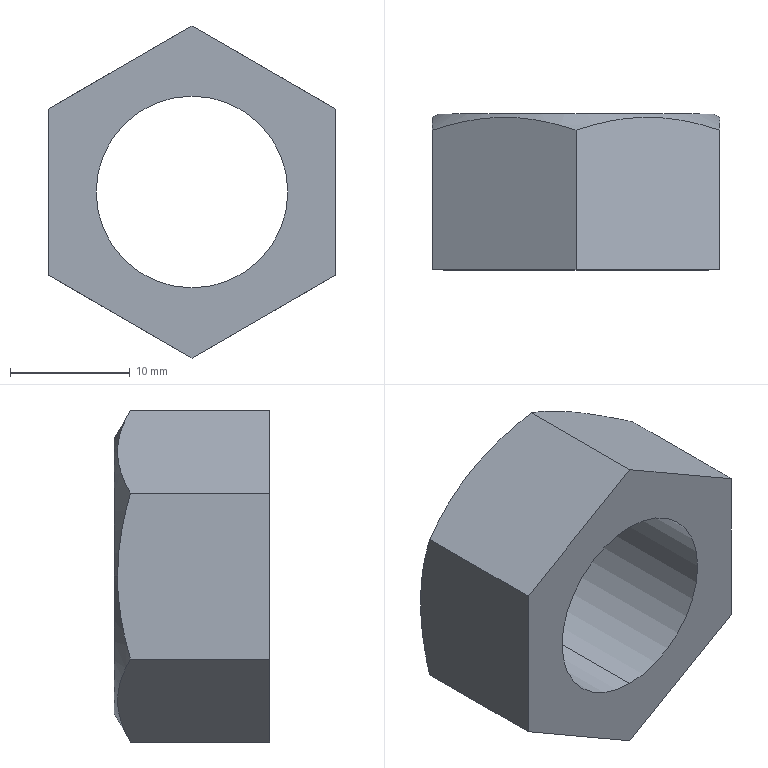Part | STEP file | NN42-M16 | 1 solid | 12 faces | box 24 x 13 x 27.713 mm | volume 3837 mm3 | plane 8 | cylinder 2 | cone 2 | commonest cylinder face diameters 16 x2
STEP:
#1=CARTESIAN_POINT('',(0.,0.,0.));
#2=DIRECTION('',(0.,0.,1.));
#3=DIRECTION('',(1.,0.,0.));
#4=AXIS2_PLACEMENT_3D('',#1,#2,#3);
#5=CARTESIAN_POINT('',(0.,13.,-8.));
#6=VERTEX_POINT('',#5);
#7=CARTESIAN_POINT('',(0.,0.,-8.));
#8=VERTEX_POINT('',#7);
#9=CARTESIAN_POINT('',(0.,13.,-8.));
#10=DIRECTION('',(0.,-1.,0.));
#11=VECTOR('',#10,1.);
#12=LINE('',#9,#11);
#13=CARTESIAN_POINT('',(0.,13.,0.));
#14=DIRECTION('',(0.,-1.,0.));
#15=DIRECTION('',(0.,0.,-1.));
#16=AXIS2_PLACEMENT_3D('',#13,#14,#15);
#17=CYLINDRICAL_SURFACE('',#16,8.);
#18=CARTESIAN_POINT('',(6.283,0.));
#19=DIRECTION('',(0.,1.));
#20=VECTOR('',#19,1.);
#21=LINE('',#18,#20);
#22=(GEOMETRIC_REPRESENTATION_CONTEXT(2)PARAMETRIC_REPRESENTATION_CONTEXT()REPRESENTATION_CONTEXT('',''));
#23=DEFINITIONAL_REPRESENTATION('',(#21),#22);
#24=PCURVE('',#17,#23);
#25=CARTESIAN_POINT('',(0.,13.,0.));
#26=DIRECTION('',(0.,-1.,0.));
#27=DIRECTION('',(0.,0.,-1.));
#28=AXIS2_PLACEMENT_3D('',#25,#26,#27);
#29=CYLINDRICAL_SURFACE('',#28,8.);
#30=CARTESIAN_POINT('',(0.,0.));
#31=DIRECTION('',(0.,1.));
#32=VECTOR('',#31,1.);
#33=LINE('',#30,#32);
#34=(GEOMETRIC_REPRESENTATION_CONTEXT(2)PARAMETRIC_REPRESENTATION_CONTEXT()REPRESENTATION_CONTEXT('',''));
#35=DEFINITIONAL_REPRESENTATION('',(#33),#34);
#36=PCURVE('',#29,#35);
#37=SURFACE_CURVE('',#12,(#24,#36),.PCURVE_S1.);
#38=EDGE_CURVE('',#6,#8,#37,.T.);
#39=ORIENTED_EDGE('',*,*,#38,.T.);
#40=CARTESIAN_POINT('',(0.,0.,8.));
#41=VERTEX_POINT('',#40);
#42=CARTESIAN_POINT('',(0.,0.,0.));
#43=DIRECTION('',(0.,1.,0.));
#44=DIRECTION('',(0.,0.,1.));
#45=AXIS2_PLACEMENT_3D('',#42,#43,#44);
#46=CIRCLE('',#45,8.);
#47=CARTESIAN_POINT('',(9.425,13.));
#48=DIRECTION('',(-1.,0.));
#49=VECTOR('',#48,1.);
#50=LINE('',#47,#49);
#51=(GEOMETRIC_REPRESENTATION_CONTEXT(2)PARAMETRIC_REPRESENTATION_CONTEXT()REPRESENTATION_CONTEXT('',''));
#52=DEFINITIONAL_REPRESENTATION('',(#50),#51);
#53=PCURVE('',#17,#52);
#54=CARTESIAN_POINT('',(0.,0.,0.));
#55=DIRECTION('',(0.,-1.,0.));
#56=DIRECTION('',(0.,0.,1.));
#57=AXIS2_PLACEMENT_3D('',#54,#55,#56);
#58=PLANE('',#57);
#59=CARTESIAN_POINT('',(8.,0.));
#60=CARTESIAN_POINT('',(8.,-13.856));
#61=CARTESIAN_POINT('',(-4.,-6.928));
#62=CARTESIAN_POINT('',(-16.,0.));
#63=CARTESIAN_POINT('',(-4.,6.928));
#64=CARTESIAN_POINT('',(8.,13.856));
#65=CARTESIAN_POINT('',(8.,0.));
#66=(BOUNDED_CURVE()B_SPLINE_CURVE(2,(#59,#60,#61,#62,#63,#64,#65),.UNSPECIFIED.,.T.,.F.)B_SPLINE_CURVE_WITH_KNOTS((1,2,2,2,2,1),(-2.094,0.,2.094,4.189,6.283,8.378),.UNSPECIFIED.)CURVE()GEOMETRIC_REPRESENTATION_ITEM()RATIONAL_B_SPLINE_CURVE((1.,0.5,1.,0.5,1.,0.5,1.))REPRESENTATION_ITEM(''));
#67=(GEOMETRIC_REPRESENTATION_CONTEXT(2)PARAMETRIC_REPRESENTATION_CONTEXT()REPRESENTATION_CONTEXT('',''));
#68=DEFINITIONAL_REPRESENTATION('',(#66),#67);
#69=PCURVE('',#58,#68);
#70=SURFACE_CURVE('',#46,(#53,#69),.PCURVE_S1.);
#71=EDGE_CURVE('',#8,#41,#70,.T.);
#72=ORIENTED_EDGE('',*,*,#71,.T.);
#73=CARTESIAN_POINT('',(0.,13.,8.));
#74=VERTEX_POINT('',#73);
#75=CARTESIAN_POINT('',(0.,13.,8.));
#76=DIRECTION('',(0.,-1.,0.));
#77=VECTOR('',#76,1.);
#78=LINE('',#75,#77);
#79=CARTESIAN_POINT('',(3.142,0.));
#80=DIRECTION('',(0.,1.));
#81=VECTOR('',#80,1.);
#82=LINE('',#79,#81);
#83=(GEOMETRIC_REPRESENTATION_CONTEXT(2)PARAMETRIC_REPRESENTATION_CONTEXT()REPRESENTATION_CONTEXT('',''));
#84=DEFINITIONAL_REPRESENTATION('',(#82),#83);
#85=PCURVE('',#17,#84);
#86=CARTESIAN_POINT('',(3.142,0.));
#87=DIRECTION('',(0.,1.));
#88=VECTOR('',#87,1.);
#89=LINE('',#86,#88);
#90=(GEOMETRIC_REPRESENTATION_CONTEXT(2)PARAMETRIC_REPRESENTATION_CONTEXT()REPRESENTATION_CONTEXT('',''));
#91=DEFINITIONAL_REPRESENTATION('',(#89),#90);
#92=PCURVE('',#29,#91);
#93=SURFACE_CURVE('',#78,(#85,#92),.PCURVE_S1.);
#94=EDGE_CURVE('',#74,#41,#93,.T.);
#95=ORIENTED_EDGE('',*,*,#94,.F.);
#96=CARTESIAN_POINT('',(0.,13.,0.));
#97=DIRECTION('',(0.,-1.,0.));
#98=DIRECTION('',(0.,0.,-1.));
#99=AXIS2_PLACEMENT_3D('',#96,#97,#98);
#100=CIRCLE('',#99,8.);
#101=CARTESIAN_POINT('',(0.,0.));
#102=DIRECTION('',(1.,0.));
#103=VECTOR('',#102,1.);
#104=LINE('',#101,#103);
#105=(GEOMETRIC_REPRESENTATION_CONTEXT(2)PARAMETRIC_REPRESENTATION_CONTEXT()REPRESENTATION_CONTEXT('',''));
#106=DEFINITIONAL_REPRESENTATION('',(#104),#105);
#107=PCURVE('',#17,#106);
#108=CARTESIAN_POINT('',(0.,13.,0.));
#109=DIRECTION('',(0.,1.,0.));
#110=DIRECTION('',(-1.,0.,0.));
#111=AXIS2_PLACEMENT_3D('',#108,#109,#110);
#112=PLANE('',#111);
#113=CARTESIAN_POINT('',(0.,-8.));
#114=CARTESIAN_POINT('',(-13.856,-8.));
#115=CARTESIAN_POINT('',(-6.928,4.));
#116=CARTESIAN_POINT('',(0.,16.));
#117=CARTESIAN_POINT('',(6.928,4.));
#118=CARTESIAN_POINT('',(13.856,-8.));
#119=CARTESIAN_POINT('',(0.,-8.));
#120=(BOUNDED_CURVE()B_SPLINE_CURVE(2,(#113,#114,#115,#116,#117,#118,#119),.UNSPECIFIED.,.T.,.F.)B_SPLINE_CURVE_WITH_KNOTS((1,2,2,2,2,1),(-2.094,0.,2.094,4.189,6.283,8.378),.UNSPECIFIED.)CURVE()GEOMETRIC_REPRESENTATION_ITEM()RATIONAL_B_SPLINE_CURVE((1.,0.5,1.,0.5,1.,0.5,1.))REPRESENTATION_ITEM(''));
#121=(GEOMETRIC_REPRESENTATION_CONTEXT(2)PARAMETRIC_REPRESENTATION_CONTEXT()REPRESENTATION_CONTEXT('',''));
#122=DEFINITIONAL_REPRESENTATION('',(#120),#121);
#123=PCURVE('',#112,#122);
#124=SURFACE_CURVE('',#100,(#107,#123),.PCURVE_S1.);
#125=EDGE_CURVE('',#74,#6,#124,.T.);
#126=ORIENTED_EDGE('',*,*,#125,.T.);
#127=EDGE_LOOP('',(#39,#72,#95,#126));
#128=FACE_BOUND('',#127,.F.);
#129=ADVANCED_FACE('',(#128),#17,.F.);
#130=CARTESIAN_POINT('',(11.5,13.,0.));
#131=VERTEX_POINT('',#130);
#132=CARTESIAN_POINT('',(-11.5,13.,0.));
#133=VERTEX_POINT('',#132);
#134=CARTESIAN_POINT('',(0.,13.,0.));
#135=DIRECTION('',(0.,-1.,0.));
#136=DIRECTION('',(1.,0.,0.));
#137=AXIS2_PLACEMENT_3D('',#134,#135,#136);
#138=CIRCLE('',#137,11.5);
#139=CARTESIAN_POINT('',(0.,13.,0.));
#140=DIRECTION('',(0.,-1.,0.));
#141=DIRECTION('',(1.,0.,0.));
#142=AXIS2_PLACEMENT_3D('',#139,#140,#141);
#143=CONICAL_SURFACE('',#142,11.5,1.047);
#144=CARTESIAN_POINT('',(0.,0.));
#145=DIRECTION('',(1.,0.));
#146=VECTOR('',#145,1.);
#147=LINE('',#144,#146);
#148=(GEOMETRIC_REPRESENTATION_CONTEXT(2)PARAMETRIC_REPRESENTATION_CONTEXT()REPRESENTATION_CONTEXT('',''));
#149=DEFINITIONAL_REPRESENTATION('',(#147),#148);
#150=PCURVE('',#143,#149);
#151=CARTESIAN_POINT('',(-11.5,0.));
#152=CARTESIAN_POINT('',(-11.5,19.919));
#153=CARTESIAN_POINT('',(5.75,9.959));
#154=CARTESIAN_POINT('',(23.,0.));
#155=CARTESIAN_POINT('',(5.75,-9.959));
#156=CARTESIAN_POINT('',(-11.5,-19.919));
#157=CARTESIAN_POINT('',(-11.5,0.));
#158=(BOUNDED_CURVE()B_SPLINE_CURVE(2,(#151,#152,#153,#154,#155,#156,#157),.UNSPECIFIED.,.T.,.F.)B_SPLINE_CURVE_WITH_KNOTS((1,2,2,2,2,1),(-2.094,0.,2.094,4.189,6.283,8.378),.UNSPECIFIED.)CURVE()GEOMETRIC_REPRESENTATION_ITEM()RATIONAL_B_SPLINE_CURVE((1.,0.5,1.,0.5,1.,0.5,1.))REPRESENTATION_ITEM(''));
#159=(GEOMETRIC_REPRESENTATION_CONTEXT(2)PARAMETRIC_REPRESENTATION_CONTEXT()REPRESENTATION_CONTEXT('',''));
#160=DEFINITIONAL_REPRESENTATION('',(#158),#159);
#161=PCURVE('',#112,#160);
#162=SURFACE_CURVE('',#138,(#150,#161),.PCURVE_S1.);
#163=EDGE_CURVE('',#131,#133,#162,.T.);
#164=ORIENTED_EDGE('',*,*,#163,.T.);
#165=CARTESIAN_POINT('',(-12.,12.711,0.));
#166=VERTEX_POINT('',#165);
#167=CARTESIAN_POINT('',(-11.5,13.,0.));
#168=DIRECTION('',(-0.866,-0.5,0.));
#169=VECTOR('',#168,1.);
#170=LINE('',#167,#169);
#171=CARTESIAN_POINT('',(3.142,0.));
#172=DIRECTION('',(0.,1.));
#173=VECTOR('',#172,1.);
#174=LINE('',#171,#173);
#175=(GEOMETRIC_REPRESENTATION_CONTEXT(2)PARAMETRIC_REPRESENTATION_CONTEXT()REPRESENTATION_CONTEXT('',''));
#176=DEFINITIONAL_REPRESENTATION('',(#174),#175);
#177=PCURVE('',#143,#176);
#178=CARTESIAN_POINT('',(0.,13.,0.));
#179=DIRECTION('',(0.,-1.,0.));
#180=DIRECTION('',(1.,0.,0.));
#181=AXIS2_PLACEMENT_3D('',#178,#179,#180);
#182=CONICAL_SURFACE('',#181,11.5,1.047);
#183=CARTESIAN_POINT('',(3.142,0.));
#184=DIRECTION('',(0.,1.));
#185=VECTOR('',#184,1.);
#186=LINE('',#183,#185);
#187=(GEOMETRIC_REPRESENTATION_CONTEXT(2)PARAMETRIC_REPRESENTATION_CONTEXT()REPRESENTATION_CONTEXT('',''));
#188=DEFINITIONAL_REPRESENTATION('',(#186),#187);
#189=PCURVE('',#182,#188);
#190=SURFACE_CURVE('',#170,(#177,#189),.PCURVE_S1.);
#191=EDGE_CURVE('',#133,#166,#190,.T.);
#192=ORIENTED_EDGE('',*,*,#191,.T.);
#193=CARTESIAN_POINT('',(-12.,11.64,6.928));
#194=VERTEX_POINT('',#193);
#195=CARTESIAN_POINT('',(-12.,11.64,6.928));
#196=CARTESIAN_POINT('',(-12.,11.965,5.8));
#197=CARTESIAN_POINT('',(-12.,12.235,4.661));
#198=CARTESIAN_POINT('',(-12.,12.608,2.355));
#199=CARTESIAN_POINT('',(-12.,12.711,1.186));
#200=CARTESIAN_POINT('',(-12.,12.711,0.));
#201=B_SPLINE_CURVE_WITH_KNOTS('',3,(#195,#196,#197,#198,#199,#200),.UNSPECIFIED.,.F.,.F.,(4,2,4),(0.01512,0.01865,0.02217),.UNSPECIFIED.);
#202=CARTESIAN_POINT('',(2.618,1.36));
#203=CARTESIAN_POINT('',(2.624,1.331));
#204=CARTESIAN_POINT('',(2.637,1.273));
#205=CARTESIAN_POINT('',(2.657,1.188));
#206=CARTESIAN_POINT('',(2.678,1.107));
#207=CARTESIAN_POINT('',(2.699,1.028));
#208=CARTESIAN_POINT('',(2.72,0.9532));
#209=CARTESIAN_POINT('',(2.742,0.8815));
#210=CARTESIAN_POINT('',(2.764,0.8133));
#211=CARTESIAN_POINT('',(2.787,0.7487));
#212=CARTESIAN_POINT('',(2.81,0.6879));
#213=CARTESIAN_POINT('',(2.833,0.6309));
#214=CARTESIAN_POINT('',(2.857,0.5779));
#215=CARTESIAN_POINT('',(2.881,0.529));
#216=CARTESIAN_POINT('',(2.906,0.4843));
#217=CARTESIAN_POINT('',(2.931,0.444));
#218=CARTESIAN_POINT('',(2.957,0.408));
#219=CARTESIAN_POINT('',(2.982,0.3766));
#220=CARTESIAN_POINT('',(3.008,0.3498));
#221=CARTESIAN_POINT('',(3.035,0.3277));
#222=CARTESIAN_POINT('',(3.061,0.3104));
#223=CARTESIAN_POINT('',(3.088,0.2979));
#224=CARTESIAN_POINT('',(3.115,0.2904));
#225=CARTESIAN_POINT('',(3.133,0.2887));
#226=CARTESIAN_POINT('',(3.142,0.2887));
#227=B_SPLINE_CURVE_WITH_KNOTS('',3,(#202,#203,#204,#205,#206,#207,#208,#209,#210,#211,#212,#213,#214,#215,#216,#217,#218,#219,#220,#221,#222,#223,#224,#225,#226),.UNSPECIFIED.,.F.,.F.,(4,1,1,1,1,1,1,1,1,1,1,1,1,1,1,1,1,1,1,1,1,1,4),(0.01512,0.01544,0.01576,0.01608,0.0164,0.01672,0.01705,0.01737,0.01769,0.01801,0.01833,0.01865,0.01897,0.01929,0.01961,0.01993,0.02025,0.02057,0.02089,0.02121,0.02153,0.02185,0.02217),.QUASI_UNIFORM_KNOTS.);
#228=(GEOMETRIC_REPRESENTATION_CONTEXT(2)PARAMETRIC_REPRESENTATION_CONTEXT()REPRESENTATION_CONTEXT('',''));
#229=DEFINITIONAL_REPRESENTATION('',(#227),#228);
#230=PCURVE('',#143,#229);
#231=CARTESIAN_POINT('',(-12.,11.64,6.928));
#232=DIRECTION('',(1.,0.,0.));
#233=DIRECTION('',(0.,0.,1.));
#234=AXIS2_PLACEMENT_3D('',#231,#232,#233);
#235=PLANE('',#234);
#236=CARTESIAN_POINT('',(0.,0.));
#237=CARTESIAN_POINT('',(-1.129,-0.3258));
#238=CARTESIAN_POINT('',(-2.267,-0.595));
#239=CARTESIAN_POINT('',(-4.574,-0.9687));
#240=CARTESIAN_POINT('',(-5.742,-1.072));
#241=CARTESIAN_POINT('',(-6.928,-1.072));
#242=B_SPLINE_CURVE_WITH_KNOTS('',3,(#236,#237,#238,#239,#240,#241),.UNSPECIFIED.,.F.,.F.,(4,2,4),(0.01512,0.01865,0.02217),.UNSPECIFIED.);
#243=(GEOMETRIC_REPRESENTATION_CONTEXT(2)PARAMETRIC_REPRESENTATION_CONTEXT()REPRESENTATION_CONTEXT('',''));
#244=DEFINITIONAL_REPRESENTATION('',(#242),#243);
#245=PCURVE('',#235,#244);
#246=SURFACE_CURVE('',#201,(#230,#245),.PCURVE_S1.);
#247=EDGE_CURVE('',#194,#166,#246,.T.);
#248=ORIENTED_EDGE('',*,*,#247,.F.);
#249=CARTESIAN_POINT('',(0.,11.64,13.856));
#250=VERTEX_POINT('',#249);
#251=CARTESIAN_POINT('',(0.,11.64,13.856));
#252=CARTESIAN_POINT('',(-0.9797,11.966,13.291));
#253=CARTESIAN_POINT('',(-1.967,12.235,12.721));
#254=CARTESIAN_POINT('',(-3.961,12.608,11.57));
#255=CARTESIAN_POINT('',(-4.968,12.711,10.988));
#256=CARTESIAN_POINT('',(-6.499,12.712,10.104));
#257=CARTESIAN_POINT('',(-7.011,12.687,9.809));
#258=CARTESIAN_POINT('',(-8.025,12.589,9.223));
#259=CARTESIAN_POINT('',(-8.528,12.516,8.933));
#260=CARTESIAN_POINT('',(-10.03,12.236,8.066));
#261=CARTESIAN_POINT('',(-11.019,11.966,7.495));
#262=CARTESIAN_POINT('',(-12.,11.64,6.928));
#263=B_SPLINE_CURVE_WITH_KNOTS('',3,(#251,#252,#253,#254,#255,#256,#257,#258,#259,#260,#261,#262),.UNSPECIFIED.,.F.,.F.,(4,2,2,2,2,4),(0.000000238,0.003499,0.006997,0.008747,0.0105,0.01399),.UNSPECIFIED.);
#264=CARTESIAN_POINT('',(1.571,1.36));
#265=CARTESIAN_POINT('',(1.584,1.301));
#266=CARTESIAN_POINT('',(1.61,1.186));
#267=CARTESIAN_POINT('',(1.651,1.026));
#268=CARTESIAN_POINT('',(1.694,0.8791));
#269=CARTESIAN_POINT('',(1.739,0.7463));
#270=CARTESIAN_POINT('',(1.786,0.6286));
#271=CARTESIAN_POINT('',(1.834,0.5268));
#272=CARTESIAN_POINT('',(1.884,0.4418));
#273=CARTESIAN_POINT('',(1.935,0.3746));
#274=CARTESIAN_POINT('',(1.987,0.3257));
#275=CARTESIAN_POINT('',(2.04,0.2957));
#276=CARTESIAN_POINT('',(2.093,0.2854));
#277=CARTESIAN_POINT('',(2.147,0.2949));
#278=CARTESIAN_POINT('',(2.2,0.3243));
#279=CARTESIAN_POINT('',(2.253,0.373));
#280=CARTESIAN_POINT('',(2.304,0.4403));
#281=CARTESIAN_POINT('',(2.354,0.5253));
#282=CARTESIAN_POINT('',(2.402,0.6273));
#283=CARTESIAN_POINT('',(2.449,0.7452));
#284=CARTESIAN_POINT('',(2.494,0.8783));
#285=CARTESIAN_POINT('',(2.537,1.026));
#286=CARTESIAN_POINT('',(2.579,1.186));
#287=CARTESIAN_POINT('',(2.605,1.301));
#288=CARTESIAN_POINT('',(2.618,1.36));
#289=B_SPLINE_CURVE_WITH_KNOTS('',3,(#264,#265,#266,#267,#268,#269,#270,#271,#272,#273,#274,#275,#276,#277,#278,#279,#280,#281,#282,#283,#284,#285,#286,#287,#288),.UNSPECIFIED.,.F.,.F.,(4,1,1,1,1,1,1,1,1,1,1,1,1,1,1,1,1,1,1,1,1,1,4),(0.000000238,0.0006363,0.001272,0.001909,0.002545,0.003181,0.003817,0.004453,0.005089,0.005725,0.006361,0.006997,0.007633,0.00827,0.008906,0.009542,0.01018,0.01081,0.01145,0.01209,0.01272,0.01336,0.01399),.QUASI_UNIFORM_KNOTS.);
#290=(GEOMETRIC_REPRESENTATION_CONTEXT(2)PARAMETRIC_REPRESENTATION_CONTEXT()REPRESENTATION_CONTEXT('',''));
#291=DEFINITIONAL_REPRESENTATION('',(#289),#290);
#292=PCURVE('',#143,#291);
#293=CARTESIAN_POINT('',(0.,11.64,13.856));
#294=DIRECTION('',(0.5,0.,-0.866));
#295=DIRECTION('',(0.866,0.,0.5));
#296=AXIS2_PLACEMENT_3D('',#293,#294,#295);
#297=PLANE('',#296);
#298=CARTESIAN_POINT('',(0.,0.));
#299=CARTESIAN_POINT('',(-1.131,-0.3266));
#300=CARTESIAN_POINT('',(-2.271,-0.5957));
#301=CARTESIAN_POINT('',(-4.573,-0.9686));
#302=CARTESIAN_POINT('',(-5.737,-1.071));
#303=CARTESIAN_POINT('',(-7.504,-1.072));
#304=CARTESIAN_POINT('',(-8.096,-1.047));
#305=CARTESIAN_POINT('',(-9.266,-0.9494));
#306=CARTESIAN_POINT('',(-9.848,-0.8769));
#307=CARTESIAN_POINT('',(-11.582,-0.5968));
#308=CARTESIAN_POINT('',(-12.724,-0.327));
#309=CARTESIAN_POINT('',(-13.856,0.));
#310=B_SPLINE_CURVE_WITH_KNOTS('',3,(#298,#299,#300,#301,#302,#303,#304,#305,#306,#307,#308,#309),.UNSPECIFIED.,.F.,.F.,(4,2,2,2,2,4),(0.000000238,0.003499,0.006997,0.008747,0.0105,0.01399),.UNSPECIFIED.);
#311=(GEOMETRIC_REPRESENTATION_CONTEXT(2)PARAMETRIC_REPRESENTATION_CONTEXT()REPRESENTATION_CONTEXT('',''));
#312=DEFINITIONAL_REPRESENTATION('',(#310),#311);
#313=PCURVE('',#297,#312);
#314=SURFACE_CURVE('',#263,(#292,#313),.PCURVE_S1.);
#315=EDGE_CURVE('',#250,#194,#314,.T.);
#316=ORIENTED_EDGE('',*,*,#315,.F.);
#317=CARTESIAN_POINT('',(12.,11.64,6.928));
#318=VERTEX_POINT('',#317);
#319=CARTESIAN_POINT('',(12.,11.64,6.928));
#320=CARTESIAN_POINT('',(11.02,11.966,7.494));
#321=CARTESIAN_POINT('',(10.033,12.235,8.064));
#322=CARTESIAN_POINT('',(8.039,12.608,9.215));
#323=CARTESIAN_POINT('',(7.032,12.711,9.797));
#324=CARTESIAN_POINT('',(5.501,12.712,10.68));
#325=CARTESIAN_POINT('',(4.989,12.687,10.976));
#326=CARTESIAN_POINT('',(3.975,12.589,11.561));
#327=CARTESIAN_POINT('',(3.472,12.516,11.852));
#328=CARTESIAN_POINT('',(1.97,12.236,12.719));
#329=CARTESIAN_POINT('',(0.9809,11.966,13.29));
#330=CARTESIAN_POINT('',(0.,11.64,13.856));
#331=B_SPLINE_CURVE_WITH_KNOTS('',3,(#319,#320,#321,#322,#323,#324,#325,#326,#327,#328,#329,#330),.UNSPECIFIED.,.F.,.F.,(4,2,2,2,2,4),(0.000000238,0.003499,0.006997,0.008747,0.0105,0.01399),.UNSPECIFIED.);
#332=CARTESIAN_POINT('',(0.5236,1.36));
#333=CARTESIAN_POINT('',(0.5365,1.301));
#334=CARTESIAN_POINT('',(0.5628,1.186));
#335=CARTESIAN_POINT('',(0.6041,1.026));
#336=CARTESIAN_POINT('',(0.6472,0.8791));
#337=CARTESIAN_POINT('',(0.6921,0.7463));
#338=CARTESIAN_POINT('',(0.7388,0.6286));
#339=CARTESIAN_POINT('',(0.787,0.5268));
#340=CARTESIAN_POINT('',(0.8367,0.4418));
#341=CARTESIAN_POINT('',(0.8877,0.3746));
#342=CARTESIAN_POINT('',(0.9397,0.3257));
#343=CARTESIAN_POINT('',(0.9926,0.2957));
#344=CARTESIAN_POINT('',(1.046,0.2854));
#345=CARTESIAN_POINT('',(1.1,0.2949));
#346=CARTESIAN_POINT('',(1.153,0.3243));
#347=CARTESIAN_POINT('',(1.205,0.373));
#348=CARTESIAN_POINT('',(1.257,0.4403));
#349=CARTESIAN_POINT('',(1.307,0.5253));
#350=CARTESIAN_POINT('',(1.355,0.6273));
#351=CARTESIAN_POINT('',(1.402,0.7452));
#352=CARTESIAN_POINT('',(1.447,0.8783));
#353=CARTESIAN_POINT('',(1.49,1.026));
#354=CARTESIAN_POINT('',(1.532,1.186));
#355=CARTESIAN_POINT('',(1.558,1.301));
#356=CARTESIAN_POINT('',(1.571,1.36));
#357=B_SPLINE_CURVE_WITH_KNOTS('',3,(#332,#333,#334,#335,#336,#337,#338,#339,#340,#341,#342,#343,#344,#345,#346,#347,#348,#349,#350,#351,#352,#353,#354,#355,#356),.UNSPECIFIED.,.F.,.F.,(4,1,1,1,1,1,1,1,1,1,1,1,1,1,1,1,1,1,1,1,1,1,4),(0.000000238,0.0006363,0.001272,0.001909,0.002545,0.003181,0.003817,0.004453,0.005089,0.005725,0.006361,0.006997,0.007633,0.00827,0.008906,0.009542,0.01018,0.01081,0.01145,0.01209,0.01272,0.01336,0.01399),.QUASI_UNIFORM_KNOTS.);
#358=(GEOMETRIC_REPRESENTATION_CONTEXT(2)PARAMETRIC_REPRESENTATION_CONTEXT()REPRESENTATION_CONTEXT('',''));
#359=DEFINITIONAL_REPRESENTATION('',(#357),#358);
#360=PCURVE('',#143,#359);
#361=CARTESIAN_POINT('',(12.,11.64,6.928));
#362=DIRECTION('',(-0.5,0.,-0.866));
#363=DIRECTION('',(0.866,0.,-0.5));
#364=AXIS2_PLACEMENT_3D('',#361,#362,#363);
#365=PLANE('',#364);
#366=CARTESIAN_POINT('',(0.,0.));
#367=CARTESIAN_POINT('',(-1.131,-0.3266));
#368=CARTESIAN_POINT('',(-2.271,-0.5957));
#369=CARTESIAN_POINT('',(-4.573,-0.9686));
#370=CARTESIAN_POINT('',(-5.737,-1.071));
#371=CARTESIAN_POINT('',(-7.504,-1.072));
#372=CARTESIAN_POINT('',(-8.096,-1.047));
#373=CARTESIAN_POINT('',(-9.266,-0.9494));
#374=CARTESIAN_POINT('',(-9.848,-0.8769));
#375=CARTESIAN_POINT('',(-11.582,-0.5968));
#376=CARTESIAN_POINT('',(-12.724,-0.327));
#377=CARTESIAN_POINT('',(-13.856,0.));
#378=B_SPLINE_CURVE_WITH_KNOTS('',3,(#366,#367,#368,#369,#370,#371,#372,#373,#374,#375,#376,#377),.UNSPECIFIED.,.F.,.F.,(4,2,2,2,2,4),(0.000000238,0.003499,0.006997,0.008747,0.0105,0.01399),.UNSPECIFIED.);
#379=(GEOMETRIC_REPRESENTATION_CONTEXT(2)PARAMETRIC_REPRESENTATION_CONTEXT()REPRESENTATION_CONTEXT('',''));
#380=DEFINITIONAL_REPRESENTATION('',(#378),#379);
#381=PCURVE('',#365,#380);
#382=SURFACE_CURVE('',#331,(#360,#381),.PCURVE_S1.);
#383=EDGE_CURVE('',#318,#250,#382,.T.);
#384=ORIENTED_EDGE('',*,*,#383,.F.);
#385=CARTESIAN_POINT('',(12.,12.711,0.));
#386=VERTEX_POINT('',#385);
#387=CARTESIAN_POINT('',(12.,12.711,0.));
#388=CARTESIAN_POINT('',(12.,12.711,1.186));
#389=CARTESIAN_POINT('',(12.,12.608,2.357));
#390=CARTESIAN_POINT('',(12.,12.234,4.663));
#391=CARTESIAN_POINT('',(12.,11.965,5.801));
#392=CARTESIAN_POINT('',(12.,11.64,6.928));
#393=B_SPLINE_CURVE_WITH_KNOTS('',3,(#387,#388,#389,#390,#391,#392),.UNSPECIFIED.,.F.,.F.,(4,2,4),(0.02217,0.02569,0.02922),.UNSPECIFIED.);
#394=CARTESIAN_POINT('',(0.,0.2887));
#395=CARTESIAN_POINT('',(0.008984,0.2887));
#396=CARTESIAN_POINT('',(0.02693,0.2904));
#397=CARTESIAN_POINT('',(0.05375,0.2979));
#398=CARTESIAN_POINT('',(0.08043,0.3104));
#399=CARTESIAN_POINT('',(0.1069,0.3277));
#400=CARTESIAN_POINT('',(0.1332,0.3499));
#401=CARTESIAN_POINT('',(0.1592,0.3767));
#402=CARTESIAN_POINT('',(0.185,0.4082));
#403=CARTESIAN_POINT('',(0.2104,0.4442));
#404=CARTESIAN_POINT('',(0.2355,0.4846));
#405=CARTESIAN_POINT('',(0.2603,0.5294));
#406=CARTESIAN_POINT('',(0.2846,0.5783));
#407=CARTESIAN_POINT('',(0.3086,0.6313));
#408=CARTESIAN_POINT('',(0.3321,0.6883));
#409=CARTESIAN_POINT('',(0.3552,0.7491));
#410=CARTESIAN_POINT('',(0.3779,0.8137));
#411=CARTESIAN_POINT('',(0.4001,0.8818));
#412=CARTESIAN_POINT('',(0.4218,0.9535));
#413=CARTESIAN_POINT('',(0.4431,1.029));
#414=CARTESIAN_POINT('',(0.464,1.107));
#415=CARTESIAN_POINT('',(0.4843,1.188));
#416=CARTESIAN_POINT('',(0.5042,1.273));
#417=CARTESIAN_POINT('',(0.5172,1.331));
#418=CARTESIAN_POINT('',(0.5236,1.36));
#419=B_SPLINE_CURVE_WITH_KNOTS('',3,(#394,#395,#396,#397,#398,#399,#400,#401,#402,#403,#404,#405,#406,#407,#408,#409,#410,#411,#412,#413,#414,#415,#416,#417,#418),.UNSPECIFIED.,.F.,.F.,(4,1,1,1,1,1,1,1,1,1,1,1,1,1,1,1,1,1,1,1,1,1,4),(0.02217,0.02249,0.02281,0.02313,0.02345,0.02377,0.02409,0.02441,0.02473,0.02505,0.02537,0.02569,0.02601,0.02633,0.02665,0.02697,0.02729,0.02762,0.02794,0.02826,0.02858,0.0289,0.02922),.QUASI_UNIFORM_KNOTS.);
#420=(GEOMETRIC_REPRESENTATION_CONTEXT(2)PARAMETRIC_REPRESENTATION_CONTEXT()REPRESENTATION_CONTEXT('',''));
#421=DEFINITIONAL_REPRESENTATION('',(#419),#420);
#422=PCURVE('',#143,#421);
#423=CARTESIAN_POINT('',(12.,11.64,-6.928));
#424=DIRECTION('',(-1.,0.,0.));
#425=DIRECTION('',(0.,0.,-1.));
#426=AXIS2_PLACEMENT_3D('',#423,#424,#425);
#427=PLANE('',#426);
#428=CARTESIAN_POINT('',(-6.928,-1.072));
#429=CARTESIAN_POINT('',(-8.114,-1.072));
#430=CARTESIAN_POINT('',(-9.285,-0.9684));
#431=CARTESIAN_POINT('',(-11.591,-0.5946));
#432=CARTESIAN_POINT('',(-12.729,-0.3254));
#433=CARTESIAN_POINT('',(-13.856,0.));
#434=B_SPLINE_CURVE_WITH_KNOTS('',3,(#428,#429,#430,#431,#432,#433),.UNSPECIFIED.,.F.,.F.,(4,2,4),(0.02217,0.02569,0.02922),.UNSPECIFIED.);
#435=(GEOMETRIC_REPRESENTATION_CONTEXT(2)PARAMETRIC_REPRESENTATION_CONTEXT()REPRESENTATION_CONTEXT('',''));
#436=DEFINITIONAL_REPRESENTATION('',(#434),#435);
#437=PCURVE('',#427,#436);
#438=SURFACE_CURVE('',#393,(#422,#437),.PCURVE_S1.);
#439=EDGE_CURVE('',#386,#318,#438,.T.);
#440=ORIENTED_EDGE('',*,*,#439,.F.);
#441=CARTESIAN_POINT('',(11.5,13.,0.));
#442=DIRECTION('',(0.866,-0.5,0.));
#443=VECTOR('',#442,1.);
#444=LINE('',#441,#443);
#445=CARTESIAN_POINT('',(0.,0.));
#446=DIRECTION('',(0.,1.));
#447=VECTOR('',#446,1.);
#448=LINE('',#445,#447);
#449=(GEOMETRIC_REPRESENTATION_CONTEXT(2)PARAMETRIC_REPRESENTATION_CONTEXT()REPRESENTATION_CONTEXT('',''));
#450=DEFINITIONAL_REPRESENTATION('',(#448),#449);
#451=PCURVE('',#143,#450);
#452=CARTESIAN_POINT('',(6.283,0.));
#453=DIRECTION('',(0.,1.));
#454=VECTOR('',#453,1.);
#455=LINE('',#452,#454);
#456=(GEOMETRIC_REPRESENTATION_CONTEXT(2)PARAMETRIC_REPRESENTATION_CONTEXT()REPRESENTATION_CONTEXT('',''));
#457=DEFINITIONAL_REPRESENTATION('',(#455),#456);
#458=PCURVE('',#182,#457);
#459=SURFACE_CURVE('',#444,(#451,#458),.PCURVE_S1.);
#460=EDGE_CURVE('',#131,#386,#459,.T.);
#461=ORIENTED_EDGE('',*,*,#460,.F.);
#462=EDGE_LOOP('',(#164,#192,#248,#316,#384,#440,#461));
#463=FACE_BOUND('',#462,.T.);
#464=ADVANCED_FACE('',(#463),#143,.T.);
#465=ORIENTED_EDGE('',*,*,#191,.F.);
#466=CARTESIAN_POINT('',(0.,13.,0.));
#467=DIRECTION('',(0.,-1.,0.));
#468=DIRECTION('',(1.,0.,0.));
#469=AXIS2_PLACEMENT_3D('',#466,#467,#468);
#470=CIRCLE('',#469,11.5);
#471=CARTESIAN_POINT('',(0.,0.));
#472=DIRECTION('',(1.,0.));
#473=VECTOR('',#472,1.);
#474=LINE('',#471,#473);
#475=(GEOMETRIC_REPRESENTATION_CONTEXT(2)PARAMETRIC_REPRESENTATION_CONTEXT()REPRESENTATION_CONTEXT('',''));
#476=DEFINITIONAL_REPRESENTATION('',(#474),#475);
#477=PCURVE('',#182,#476);
#478=CARTESIAN_POINT('',(-11.5,0.));
#479=CARTESIAN_POINT('',(-11.5,19.919));
#480=CARTESIAN_POINT('',(5.75,9.959));
#481=CARTESIAN_POINT('',(23.,0.));
#482=CARTESIAN_POINT('',(5.75,-9.959));
#483=CARTESIAN_POINT('',(-11.5,-19.919));
#484=CARTESIAN_POINT('',(-11.5,0.));
#485=(BOUNDED_CURVE()B_SPLINE_CURVE(2,(#478,#479,#480,#481,#482,#483,#484),.UNSPECIFIED.,.T.,.F.)B_SPLINE_CURVE_WITH_KNOTS((1,2,2,2,2,1),(-2.094,0.,2.094,4.189,6.283,8.378),.UNSPECIFIED.)CURVE()GEOMETRIC_REPRESENTATION_ITEM()RATIONAL_B_SPLINE_CURVE((1.,0.5,1.,0.5,1.,0.5,1.))REPRESENTATION_ITEM(''));
#486=(GEOMETRIC_REPRESENTATION_CONTEXT(2)PARAMETRIC_REPRESENTATION_CONTEXT()REPRESENTATION_CONTEXT('',''));
#487=DEFINITIONAL_REPRESENTATION('',(#485),#486);
#488=PCURVE('',#112,#487);
#489=SURFACE_CURVE('',#470,(#477,#488),.PCURVE_S1.);
#490=EDGE_CURVE('',#133,#131,#489,.T.);
#491=ORIENTED_EDGE('',*,*,#490,.T.);
#492=ORIENTED_EDGE('',*,*,#460,.T.);
#493=CARTESIAN_POINT('',(12.,11.64,-6.928));
#494=VERTEX_POINT('',#493);
#495=CARTESIAN_POINT('',(12.,11.64,-6.928));
#496=CARTESIAN_POINT('',(12.,11.965,-5.8));
#497=CARTESIAN_POINT('',(12.,12.235,-4.661));
#498=CARTESIAN_POINT('',(12.,12.608,-2.355));
#499=CARTESIAN_POINT('',(12.,12.711,-1.186));
#500=CARTESIAN_POINT('',(12.,12.711,0.));
#501=B_SPLINE_CURVE_WITH_KNOTS('',3,(#495,#496,#497,#498,#499,#500),.UNSPECIFIED.,.F.,.F.,(4,2,4),(0.01512,0.01865,0.02217),.UNSPECIFIED.);
#502=CARTESIAN_POINT('',(5.76,1.36));
#503=CARTESIAN_POINT('',(5.766,1.331));
#504=CARTESIAN_POINT('',(5.779,1.273));
#505=CARTESIAN_POINT('',(5.799,1.188));
#506=CARTESIAN_POINT('',(5.819,1.107));
#507=CARTESIAN_POINT('',(5.84,1.028));
#508=CARTESIAN_POINT('',(5.861,0.9532));
#509=CARTESIAN_POINT('',(5.883,0.8815));
#510=CARTESIAN_POINT('',(5.905,0.8133));
#511=CARTESIAN_POINT('',(5.928,0.7487));
#512=CARTESIAN_POINT('',(5.951,0.6879));
#513=CARTESIAN_POINT('',(5.975,0.6309));
#514=CARTESIAN_POINT('',(5.999,0.5779));
#515=CARTESIAN_POINT('',(6.023,0.529));
#516=CARTESIAN_POINT('',(6.048,0.4843));
#517=CARTESIAN_POINT('',(6.073,0.444));
#518=CARTESIAN_POINT('',(6.098,0.408));
#519=CARTESIAN_POINT('',(6.124,0.3766));
#520=CARTESIAN_POINT('',(6.15,0.3498));
#521=CARTESIAN_POINT('',(6.176,0.3277));
#522=CARTESIAN_POINT('',(6.203,0.3104));
#523=CARTESIAN_POINT('',(6.229,0.2979));
#524=CARTESIAN_POINT('',(6.256,0.2904));
#525=CARTESIAN_POINT('',(6.274,0.2887));
#526=CARTESIAN_POINT('',(6.283,0.2887));
#527=B_SPLINE_CURVE_WITH_KNOTS('',3,(#502,#503,#504,#505,#506,#507,#508,#509,#510,#511,#512,#513,#514,#515,#516,#517,#518,#519,#520,#521,#522,#523,#524,#525,#526),.UNSPECIFIED.,.F.,.F.,(4,1,1,1,1,1,1,1,1,1,1,1,1,1,1,1,1,1,1,1,1,1,4),(0.01512,0.01544,0.01576,0.01608,0.0164,0.01672,0.01705,0.01737,0.01769,0.01801,0.01833,0.01865,0.01897,0.01929,0.01961,0.01993,0.02025,0.02057,0.02089,0.02121,0.02153,0.02185,0.02217),.QUASI_UNIFORM_KNOTS.);
#528=(GEOMETRIC_REPRESENTATION_CONTEXT(2)PARAMETRIC_REPRESENTATION_CONTEXT()REPRESENTATION_CONTEXT('',''));
#529=DEFINITIONAL_REPRESENTATION('',(#527),#528);
#530=PCURVE('',#182,#529);
#531=CARTESIAN_POINT('',(0.,0.));
#532=CARTESIAN_POINT('',(-1.129,-0.3258));
#533=CARTESIAN_POINT('',(-2.267,-0.595));
#534=CARTESIAN_POINT('',(-4.574,-0.9687));
#535=CARTESIAN_POINT('',(-5.742,-1.072));
#536=CARTESIAN_POINT('',(-6.928,-1.072));
#537=B_SPLINE_CURVE_WITH_KNOTS('',3,(#531,#532,#533,#534,#535,#536),.UNSPECIFIED.,.F.,.F.,(4,2,4),(0.01512,0.01865,0.02217),.UNSPECIFIED.);
#538=(GEOMETRIC_REPRESENTATION_CONTEXT(2)PARAMETRIC_REPRESENTATION_CONTEXT()REPRESENTATION_CONTEXT('',''));
#539=DEFINITIONAL_REPRESENTATION('',(#537),#538);
#540=PCURVE('',#427,#539);
#541=SURFACE_CURVE('',#501,(#530,#540),.PCURVE_S1.);
#542=EDGE_CURVE('',#494,#386,#541,.T.);
#543=ORIENTED_EDGE('',*,*,#542,.F.);
#544=CARTESIAN_POINT('',(0.,11.64,-13.856));
#545=VERTEX_POINT('',#544);
#546=CARTESIAN_POINT('',(0.,11.64,-13.856));
#547=CARTESIAN_POINT('',(0.9797,11.966,-13.291));
#548=CARTESIAN_POINT('',(1.967,12.235,-12.721));
#549=CARTESIAN_POINT('',(3.961,12.608,-11.57));
#550=CARTESIAN_POINT('',(4.968,12.711,-10.988));
#551=CARTESIAN_POINT('',(6.499,12.712,-10.104));
#552=CARTESIAN_POINT('',(7.011,12.687,-9.809));
#553=CARTESIAN_POINT('',(8.025,12.589,-9.223));
#554=CARTESIAN_POINT('',(8.528,12.516,-8.933));
#555=CARTESIAN_POINT('',(10.03,12.236,-8.066));
#556=CARTESIAN_POINT('',(11.019,11.966,-7.495));
#557=CARTESIAN_POINT('',(12.,11.64,-6.928));
#558=B_SPLINE_CURVE_WITH_KNOTS('',3,(#546,#547,#548,#549,#550,#551,#552,#553,#554,#555,#556,#557),.UNSPECIFIED.,.F.,.F.,(4,2,2,2,2,4),(0.000000238,0.003499,0.006997,0.008747,0.0105,0.01399),.UNSPECIFIED.);
#559=CARTESIAN_POINT('',(4.712,1.36));
#560=CARTESIAN_POINT('',(4.725,1.301));
#561=CARTESIAN_POINT('',(4.752,1.186));
#562=CARTESIAN_POINT('',(4.793,1.026));
#563=CARTESIAN_POINT('',(4.836,0.8791));
#564=CARTESIAN_POINT('',(4.881,0.7463));
#565=CARTESIAN_POINT('',(4.928,0.6286));
#566=CARTESIAN_POINT('',(4.976,0.5268));
#567=CARTESIAN_POINT('',(5.025,0.4418));
#568=CARTESIAN_POINT('',(5.076,0.3746));
#569=CARTESIAN_POINT('',(5.129,0.3257));
#570=CARTESIAN_POINT('',(5.181,0.2957));
#571=CARTESIAN_POINT('',(5.235,0.2854));
#572=CARTESIAN_POINT('',(5.288,0.2949));
#573=CARTESIAN_POINT('',(5.342,0.3243));
#574=CARTESIAN_POINT('',(5.394,0.373));
#575=CARTESIAN_POINT('',(5.445,0.4403));
#576=CARTESIAN_POINT('',(5.495,0.5253));
#577=CARTESIAN_POINT('',(5.544,0.6273));
#578=CARTESIAN_POINT('',(5.591,0.7452));
#579=CARTESIAN_POINT('',(5.636,0.8783));
#580=CARTESIAN_POINT('',(5.679,1.026));
#581=CARTESIAN_POINT('',(5.72,1.186));
#582=CARTESIAN_POINT('',(5.747,1.301));
#583=CARTESIAN_POINT('',(5.76,1.36));
#584=B_SPLINE_CURVE_WITH_KNOTS('',3,(#559,#560,#561,#562,#563,#564,#565,#566,#567,#568,#569,#570,#571,#572,#573,#574,#575,#576,#577,#578,#579,#580,#581,#582,#583),.UNSPECIFIED.,.F.,.F.,(4,1,1,1,1,1,1,1,1,1,1,1,1,1,1,1,1,1,1,1,1,1,4),(0.000000238,0.0006363,0.001272,0.001909,0.002545,0.003181,0.003817,0.004453,0.005089,0.005725,0.006361,0.006997,0.007633,0.00827,0.008906,0.009542,0.01018,0.01081,0.01145,0.01209,0.01272,0.01336,0.01399),.QUASI_UNIFORM_KNOTS.);
#585=(GEOMETRIC_REPRESENTATION_CONTEXT(2)PARAMETRIC_REPRESENTATION_CONTEXT()REPRESENTATION_CONTEXT('',''));
#586=DEFINITIONAL_REPRESENTATION('',(#584),#585);
#587=PCURVE('',#182,#586);
#588=CARTESIAN_POINT('',(0.,11.64,-13.856));
#589=DIRECTION('',(-0.5,0.,0.866));
#590=DIRECTION('',(-0.866,0.,-0.5));
#591=AXIS2_PLACEMENT_3D('',#588,#589,#590);
#592=PLANE('',#591);
#593=CARTESIAN_POINT('',(0.,0.));
#594=CARTESIAN_POINT('',(-1.131,-0.3266));
#595=CARTESIAN_POINT('',(-2.271,-0.5957));
#596=CARTESIAN_POINT('',(-4.573,-0.9686));
#597=CARTESIAN_POINT('',(-5.737,-1.071));
#598=CARTESIAN_POINT('',(-7.504,-1.072));
#599=CARTESIAN_POINT('',(-8.096,-1.047));
#600=CARTESIAN_POINT('',(-9.266,-0.9494));
#601=CARTESIAN_POINT('',(-9.848,-0.8769));
#602=CARTESIAN_POINT('',(-11.582,-0.5968));
#603=CARTESIAN_POINT('',(-12.724,-0.327));
#604=CARTESIAN_POINT('',(-13.856,0.));
#605=B_SPLINE_CURVE_WITH_KNOTS('',3,(#593,#594,#595,#596,#597,#598,#599,#600,#601,#602,#603,#604),.UNSPECIFIED.,.F.,.F.,(4,2,2,2,2,4),(0.000000238,0.003499,0.006997,0.008747,0.0105,0.01399),.UNSPECIFIED.);
#606=(GEOMETRIC_REPRESENTATION_CONTEXT(2)PARAMETRIC_REPRESENTATION_CONTEXT()REPRESENTATION_CONTEXT('',''));
#607=DEFINITIONAL_REPRESENTATION('',(#605),#606);
#608=PCURVE('',#592,#607);
#609=SURFACE_CURVE('',#558,(#587,#608),.PCURVE_S1.);
#610=EDGE_CURVE('',#545,#494,#609,.T.);
#611=ORIENTED_EDGE('',*,*,#610,.F.);
#612=CARTESIAN_POINT('',(-12.,11.64,-6.928));
#613=VERTEX_POINT('',#612);
#614=CARTESIAN_POINT('',(-12.,11.64,-6.928));
#615=CARTESIAN_POINT('',(-11.02,11.966,-7.494));
#616=CARTESIAN_POINT('',(-10.033,12.235,-8.064));
#617=CARTESIAN_POINT('',(-8.039,12.608,-9.215));
#618=CARTESIAN_POINT('',(-7.032,12.711,-9.797));
#619=CARTESIAN_POINT('',(-5.501,12.712,-10.68));
#620=CARTESIAN_POINT('',(-4.989,12.687,-10.976));
#621=CARTESIAN_POINT('',(-3.975,12.589,-11.561));
#622=CARTESIAN_POINT('',(-3.472,12.516,-11.852));
#623=CARTESIAN_POINT('',(-1.97,12.236,-12.719));
#624=CARTESIAN_POINT('',(-0.9809,11.966,-13.29));
#625=CARTESIAN_POINT('',(0.,11.64,-13.856));
#626=B_SPLINE_CURVE_WITH_KNOTS('',3,(#614,#615,#616,#617,#618,#619,#620,#621,#622,#623,#624,#625),.UNSPECIFIED.,.F.,.F.,(4,2,2,2,2,4),(0.000000238,0.003499,0.006997,0.008747,0.0105,0.01399),.UNSPECIFIED.);
#627=CARTESIAN_POINT('',(3.665,1.36));
#628=CARTESIAN_POINT('',(3.678,1.301));
#629=CARTESIAN_POINT('',(3.704,1.186));
#630=CARTESIAN_POINT('',(3.746,1.026));
#631=CARTESIAN_POINT('',(3.789,0.8791));
#632=CARTESIAN_POINT('',(3.834,0.7463));
#633=CARTESIAN_POINT('',(3.88,0.6286));
#634=CARTESIAN_POINT('',(3.929,0.5268));
#635=CARTESIAN_POINT('',(3.978,0.4418));
#636=CARTESIAN_POINT('',(4.029,0.3746));
#637=CARTESIAN_POINT('',(4.081,0.3257));
#638=CARTESIAN_POINT('',(4.134,0.2957));
#639=CARTESIAN_POINT('',(4.188,0.2854));
#640=CARTESIAN_POINT('',(4.241,0.2949));
#641=CARTESIAN_POINT('',(4.295,0.3243));
#642=CARTESIAN_POINT('',(4.347,0.373));
#643=CARTESIAN_POINT('',(4.398,0.4403));
#644=CARTESIAN_POINT('',(4.448,0.5253));
#645=CARTESIAN_POINT('',(4.497,0.6273));
#646=CARTESIAN_POINT('',(4.543,0.7452));
#647=CARTESIAN_POINT('',(4.589,0.8783));
#648=CARTESIAN_POINT('',(4.632,1.026));
#649=CARTESIAN_POINT('',(4.673,1.186));
#650=CARTESIAN_POINT('',(4.7,1.301));
#651=CARTESIAN_POINT('',(4.712,1.36));
#652=B_SPLINE_CURVE_WITH_KNOTS('',3,(#627,#628,#629,#630,#631,#632,#633,#634,#635,#636,#637,#638,#639,#640,#641,#642,#643,#644,#645,#646,#647,#648,#649,#650,#651),.UNSPECIFIED.,.F.,.F.,(4,1,1,1,1,1,1,1,1,1,1,1,1,1,1,1,1,1,1,1,1,1,4),(0.000000238,0.0006363,0.001272,0.001909,0.002545,0.003181,0.003817,0.004453,0.005089,0.005725,0.006361,0.006997,0.007633,0.00827,0.008906,0.009542,0.01018,0.01081,0.01145,0.01209,0.01272,0.01336,0.01399),.QUASI_UNIFORM_KNOTS.);
#653=(GEOMETRIC_REPRESENTATION_CONTEXT(2)PARAMETRIC_REPRESENTATION_CONTEXT()REPRESENTATION_CONTEXT('',''));
#654=DEFINITIONAL_REPRESENTATION('',(#652),#653);
#655=PCURVE('',#182,#654);
#656=CARTESIAN_POINT('',(-12.,11.64,-6.928));
#657=DIRECTION('',(0.5,0.,0.866));
#658=DIRECTION('',(-0.866,0.,0.5));
#659=AXIS2_PLACEMENT_3D('',#656,#657,#658);
#660=PLANE('',#659);
#661=CARTESIAN_POINT('',(0.,0.));
#662=CARTESIAN_POINT('',(-1.131,-0.3266));
#663=CARTESIAN_POINT('',(-2.271,-0.5957));
#664=CARTESIAN_POINT('',(-4.573,-0.9686));
#665=CARTESIAN_POINT('',(-5.737,-1.071));
#666=CARTESIAN_POINT('',(-7.504,-1.072));
#667=CARTESIAN_POINT('',(-8.096,-1.047));
#668=CARTESIAN_POINT('',(-9.266,-0.9494));
#669=CARTESIAN_POINT('',(-9.848,-0.8769));
#670=CARTESIAN_POINT('',(-11.582,-0.5968));
#671=CARTESIAN_POINT('',(-12.724,-0.327));
#672=CARTESIAN_POINT('',(-13.856,0.));
#673=B_SPLINE_CURVE_WITH_KNOTS('',3,(#661,#662,#663,#664,#665,#666,#667,#668,#669,#670,#671,#672),.UNSPECIFIED.,.F.,.F.,(4,2,2,2,2,4),(0.000000238,0.003499,0.006997,0.008747,0.0105,0.01399),.UNSPECIFIED.);
#674=(GEOMETRIC_REPRESENTATION_CONTEXT(2)PARAMETRIC_REPRESENTATION_CONTEXT()REPRESENTATION_CONTEXT('',''));
#675=DEFINITIONAL_REPRESENTATION('',(#673),#674);
#676=PCURVE('',#660,#675);
#677=SURFACE_CURVE('',#626,(#655,#676),.PCURVE_S1.);
#678=EDGE_CURVE('',#613,#545,#677,.T.);
#679=ORIENTED_EDGE('',*,*,#678,.F.);
#680=CARTESIAN_POINT('',(-12.,12.711,0.));
#681=CARTESIAN_POINT('',(-12.,12.711,-1.186));
#682=CARTESIAN_POINT('',(-12.,12.608,-2.357));
#683=CARTESIAN_POINT('',(-12.,12.234,-4.663));
#684=CARTESIAN_POINT('',(-12.,11.965,-5.801));
#685=CARTESIAN_POINT('',(-12.,11.64,-6.928));
#686=B_SPLINE_CURVE_WITH_KNOTS('',3,(#680,#681,#682,#683,#684,#685),.UNSPECIFIED.,.F.,.F.,(4,2,4),(0.02217,0.02569,0.02922),.UNSPECIFIED.);
#687=CARTESIAN_POINT('',(3.142,0.2887));
#688=CARTESIAN_POINT('',(3.151,0.2887));
#689=CARTESIAN_POINT('',(3.169,0.2904));
#690=CARTESIAN_POINT('',(3.195,0.2979));
#691=CARTESIAN_POINT('',(3.222,0.3104));
#692=CARTESIAN_POINT('',(3.249,0.3277));
#693=CARTESIAN_POINT('',(3.275,0.3499));
#694=CARTESIAN_POINT('',(3.301,0.3767));
#695=CARTESIAN_POINT('',(3.327,0.4082));
#696=CARTESIAN_POINT('',(3.352,0.4442));
#697=CARTESIAN_POINT('',(3.377,0.4846));
#698=CARTESIAN_POINT('',(3.402,0.5294));
#699=CARTESIAN_POINT('',(3.426,0.5783));
#700=CARTESIAN_POINT('',(3.45,0.6313));
#701=CARTESIAN_POINT('',(3.474,0.6883));
#702=CARTESIAN_POINT('',(3.497,0.7491));
#703=CARTESIAN_POINT('',(3.519,0.8137));
#704=CARTESIAN_POINT('',(3.542,0.8818));
#705=CARTESIAN_POINT('',(3.563,0.9535));
#706=CARTESIAN_POINT('',(3.585,1.029));
#707=CARTESIAN_POINT('',(3.606,1.107));
#708=CARTESIAN_POINT('',(3.626,1.188));
#709=CARTESIAN_POINT('',(3.646,1.273));
#710=CARTESIAN_POINT('',(3.659,1.331));
#711=CARTESIAN_POINT('',(3.665,1.36));
#712=B_SPLINE_CURVE_WITH_KNOTS('',3,(#687,#688,#689,#690,#691,#692,#693,#694,#695,#696,#697,#698,#699,#700,#701,#702,#703,#704,#705,#706,#707,#708,#709,#710,#711),.UNSPECIFIED.,.F.,.F.,(4,1,1,1,1,1,1,1,1,1,1,1,1,1,1,1,1,1,1,1,1,1,4),(0.02217,0.02249,0.02281,0.02313,0.02345,0.02377,0.02409,0.02441,0.02473,0.02505,0.02537,0.02569,0.02601,0.02633,0.02665,0.02697,0.02729,0.02762,0.02794,0.02826,0.02858,0.0289,0.02922),.QUASI_UNIFORM_KNOTS.);
#713=(GEOMETRIC_REPRESENTATION_CONTEXT(2)PARAMETRIC_REPRESENTATION_CONTEXT()REPRESENTATION_CONTEXT('',''));
#714=DEFINITIONAL_REPRESENTATION('',(#712),#713);
#715=PCURVE('',#182,#714);
#716=CARTESIAN_POINT('',(-6.928,-1.072));
#717=CARTESIAN_POINT('',(-8.114,-1.072));
#718=CARTESIAN_POINT('',(-9.285,-0.9684));
#719=CARTESIAN_POINT('',(-11.591,-0.5946));
#720=CARTESIAN_POINT('',(-12.729,-0.3254));
#721=CARTESIAN_POINT('',(-13.856,0.));
#722=B_SPLINE_CURVE_WITH_KNOTS('',3,(#716,#717,#718,#719,#720,#721),.UNSPECIFIED.,.F.,.F.,(4,2,4),(0.02217,0.02569,0.02922),.UNSPECIFIED.);
#723=(GEOMETRIC_REPRESENTATION_CONTEXT(2)PARAMETRIC_REPRESENTATION_CONTEXT()REPRESENTATION_CONTEXT('',''));
#724=DEFINITIONAL_REPRESENTATION('',(#722),#723);
#725=PCURVE('',#235,#724);
#726=SURFACE_CURVE('',#686,(#715,#725),.PCURVE_S1.);
#727=EDGE_CURVE('',#166,#613,#726,.T.);
#728=ORIENTED_EDGE('',*,*,#727,.F.);
#729=EDGE_LOOP('',(#465,#491,#492,#543,#611,#679,#728));
#730=FACE_BOUND('',#729,.T.);
#731=ADVANCED_FACE('',(#730),#182,.T.);
#732=CARTESIAN_POINT('',(0.,13.,0.));
#733=DIRECTION('',(0.,-1.,0.));
#734=DIRECTION('',(0.,0.,-1.));
#735=AXIS2_PLACEMENT_3D('',#732,#733,#734);
#736=CIRCLE('',#735,8.);
#737=CARTESIAN_POINT('',(0.,-8.));
#738=CARTESIAN_POINT('',(-13.856,-8.));
#739=CARTESIAN_POINT('',(-6.928,4.));
#740=CARTESIAN_POINT('',(0.,16.));
#741=CARTESIAN_POINT('',(6.928,4.));
#742=CARTESIAN_POINT('',(13.856,-8.));
#743=CARTESIAN_POINT('',(0.,-8.));
#744=(BOUNDED_CURVE()B_SPLINE_CURVE(2,(#737,#738,#739,#740,#741,#742,#743),.UNSPECIFIED.,.T.,.F.)B_SPLINE_CURVE_WITH_KNOTS((1,2,2,2,2,1),(-2.094,0.,2.094,4.189,6.283,8.378),.UNSPECIFIED.)CURVE()GEOMETRIC_REPRESENTATION_ITEM()RATIONAL_B_SPLINE_CURVE((1.,0.5,1.,0.5,1.,0.5,1.))REPRESENTATION_ITEM(''));
#745=(GEOMETRIC_REPRESENTATION_CONTEXT(2)PARAMETRIC_REPRESENTATION_CONTEXT()REPRESENTATION_CONTEXT('',''));
#746=DEFINITIONAL_REPRESENTATION('',(#744),#745);
#747=PCURVE('',#112,#746);
#748=CARTESIAN_POINT('',(0.,0.));
#749=DIRECTION('',(1.,0.));
#750=VECTOR('',#749,1.);
#751=LINE('',#748,#750);
#752=(GEOMETRIC_REPRESENTATION_CONTEXT(2)PARAMETRIC_REPRESENTATION_CONTEXT()REPRESENTATION_CONTEXT('',''));
#753=DEFINITIONAL_REPRESENTATION('',(#751),#752);
#754=PCURVE('',#29,#753);
#755=SURFACE_CURVE('',#736,(#747,#754),.PCURVE_S1.);
#756=EDGE_CURVE('',#6,#74,#755,.T.);
#757=ORIENTED_EDGE('',*,*,#756,.T.);
#758=ORIENTED_EDGE('',*,*,#125,.T.);
#759=EDGE_LOOP('',(#757,#758));
#760=FACE_BOUND('',#759,.T.);
#761=ORIENTED_EDGE('',*,*,#163,.F.);
#762=ORIENTED_EDGE('',*,*,#490,.F.);
#763=EDGE_LOOP('',(#761,#762));
#764=FACE_BOUND('',#763,.T.);
#765=ADVANCED_FACE('',(#760,#764),#112,.T.);
#766=ORIENTED_EDGE('',*,*,#542,.T.);
#767=ORIENTED_EDGE('',*,*,#439,.T.);
#768=CARTESIAN_POINT('',(12.,0.,6.928));
#769=VERTEX_POINT('',#768);
#770=CARTESIAN_POINT('',(12.,0.,6.928));
#771=DIRECTION('',(0.,1.,0.));
#772=VECTOR('',#771,1.);
#773=LINE('',#770,#772);
#774=CARTESIAN_POINT('',(-13.856,11.64));
#775=DIRECTION('',(0.,-1.));
#776=VECTOR('',#775,1.);
#777=LINE('',#774,#776);
#778=(GEOMETRIC_REPRESENTATION_CONTEXT(2)PARAMETRIC_REPRESENTATION_CONTEXT()REPRESENTATION_CONTEXT('',''));
#779=DEFINITIONAL_REPRESENTATION('',(#777),#778);
#780=PCURVE('',#427,#779);
#781=CARTESIAN_POINT('',(0.,11.64));
#782=DIRECTION('',(0.,-1.));
#783=VECTOR('',#782,1.);
#784=LINE('',#781,#783);
#785=(GEOMETRIC_REPRESENTATION_CONTEXT(2)PARAMETRIC_REPRESENTATION_CONTEXT()REPRESENTATION_CONTEXT('',''));
#786=DEFINITIONAL_REPRESENTATION('',(#784),#785);
#787=PCURVE('',#365,#786);
#788=SURFACE_CURVE('',#773,(#780,#787),.PCURVE_S1.);
#789=EDGE_CURVE('',#769,#318,#788,.T.);
#790=ORIENTED_EDGE('',*,*,#789,.F.);
#791=CARTESIAN_POINT('',(12.,0.,-6.928));
#792=VERTEX_POINT('',#791);
#793=CARTESIAN_POINT('',(12.,0.,-6.928));
#794=DIRECTION('',(0.,0.,1.));
#795=VECTOR('',#794,1.);
#796=LINE('',#793,#795);
#797=CARTESIAN_POINT('',(0.,11.64));
#798=DIRECTION('',(-1.,0.));
#799=VECTOR('',#798,1.);
#800=LINE('',#797,#799);
#801=(GEOMETRIC_REPRESENTATION_CONTEXT(2)PARAMETRIC_REPRESENTATION_CONTEXT()REPRESENTATION_CONTEXT('',''));
#802=DEFINITIONAL_REPRESENTATION('',(#800),#801);
#803=PCURVE('',#427,#802);
#804=CARTESIAN_POINT('',(-6.928,-12.));
#805=DIRECTION('',(1.,0.));
#806=VECTOR('',#805,1.);
#807=LINE('',#804,#806);
#808=(GEOMETRIC_REPRESENTATION_CONTEXT(2)PARAMETRIC_REPRESENTATION_CONTEXT()REPRESENTATION_CONTEXT('',''));
#809=DEFINITIONAL_REPRESENTATION('',(#807),#808);
#810=PCURVE('',#58,#809);
#811=SURFACE_CURVE('',#796,(#803,#810),.PCURVE_S1.);
#812=EDGE_CURVE('',#792,#769,#811,.T.);
#813=ORIENTED_EDGE('',*,*,#812,.F.);
#814=CARTESIAN_POINT('',(12.,0.,-6.928));
#815=DIRECTION('',(0.,1.,0.));
#816=VECTOR('',#815,1.);
#817=LINE('',#814,#816);
#818=CARTESIAN_POINT('',(0.,11.64));
#819=DIRECTION('',(0.,-1.));
#820=VECTOR('',#819,1.);
#821=LINE('',#818,#820);
#822=(GEOMETRIC_REPRESENTATION_CONTEXT(2)PARAMETRIC_REPRESENTATION_CONTEXT()REPRESENTATION_CONTEXT('',''));
#823=DEFINITIONAL_REPRESENTATION('',(#821),#822);
#824=PCURVE('',#427,#823);
#825=CARTESIAN_POINT('',(-13.856,11.64));
#826=DIRECTION('',(0.,-1.));
#827=VECTOR('',#826,1.);
#828=LINE('',#825,#827);
#829=(GEOMETRIC_REPRESENTATION_CONTEXT(2)PARAMETRIC_REPRESENTATION_CONTEXT()REPRESENTATION_CONTEXT('',''));
#830=DEFINITIONAL_REPRESENTATION('',(#828),#829);
#831=PCURVE('',#592,#830);
#832=SURFACE_CURVE('',#817,(#824,#831),.PCURVE_S1.);
#833=EDGE_CURVE('',#792,#494,#832,.T.);
#834=ORIENTED_EDGE('',*,*,#833,.T.);
#835=EDGE_LOOP('',(#766,#767,#790,#813,#834));
#836=FACE_BOUND('',#835,.T.);
#837=ADVANCED_FACE('',(#836),#427,.F.);
#838=ORIENTED_EDGE('',*,*,#610,.T.);
#839=ORIENTED_EDGE('',*,*,#833,.F.);
#840=CARTESIAN_POINT('',(0.,0.,-13.856));
#841=VERTEX_POINT('',#840);
#842=CARTESIAN_POINT('',(0.,0.,-13.856));
#843=DIRECTION('',(0.866,0.,0.5));
#844=VECTOR('',#843,1.);
#845=LINE('',#842,#844);
#846=CARTESIAN_POINT('',(0.,11.64));
#847=DIRECTION('',(-1.,0.));
#848=VECTOR('',#847,1.);
#849=LINE('',#846,#848);
#850=(GEOMETRIC_REPRESENTATION_CONTEXT(2)PARAMETRIC_REPRESENTATION_CONTEXT()REPRESENTATION_CONTEXT('',''));
#851=DEFINITIONAL_REPRESENTATION('',(#849),#850);
#852=PCURVE('',#592,#851);
#853=CARTESIAN_POINT('',(-13.856,0.));
#854=DIRECTION('',(0.5,-0.866));
#855=VECTOR('',#854,1.);
#856=LINE('',#853,#855);
#857=(GEOMETRIC_REPRESENTATION_CONTEXT(2)PARAMETRIC_REPRESENTATION_CONTEXT()REPRESENTATION_CONTEXT('',''));
#858=DEFINITIONAL_REPRESENTATION('',(#856),#857);
#859=PCURVE('',#58,#858);
#860=SURFACE_CURVE('',#845,(#852,#859),.PCURVE_S1.);
#861=EDGE_CURVE('',#841,#792,#860,.T.);
#862=ORIENTED_EDGE('',*,*,#861,.F.);
#863=CARTESIAN_POINT('',(0.,0.,-13.856));
#864=DIRECTION('',(0.,1.,0.));
#865=VECTOR('',#864,1.);
#866=LINE('',#863,#865);
#867=CARTESIAN_POINT('',(0.,11.64));
#868=DIRECTION('',(0.,-1.));
#869=VECTOR('',#868,1.);
#870=LINE('',#867,#869);
#871=(GEOMETRIC_REPRESENTATION_CONTEXT(2)PARAMETRIC_REPRESENTATION_CONTEXT()REPRESENTATION_CONTEXT('',''));
#872=DEFINITIONAL_REPRESENTATION('',(#870),#871);
#873=PCURVE('',#592,#872);
#874=CARTESIAN_POINT('',(-13.856,11.64));
#875=DIRECTION('',(0.,-1.));
#876=VECTOR('',#875,1.);
#877=LINE('',#874,#876);
#878=(GEOMETRIC_REPRESENTATION_CONTEXT(2)PARAMETRIC_REPRESENTATION_CONTEXT()REPRESENTATION_CONTEXT('',''));
#879=DEFINITIONAL_REPRESENTATION('',(#877),#878);
#880=PCURVE('',#660,#879);
#881=SURFACE_CURVE('',#866,(#873,#880),.PCURVE_S1.);
#882=EDGE_CURVE('',#841,#545,#881,.T.);
#883=ORIENTED_EDGE('',*,*,#882,.T.);
#884=EDGE_LOOP('',(#838,#839,#862,#883));
#885=FACE_BOUND('',#884,.T.);
#886=ADVANCED_FACE('',(#885),#592,.F.);
#887=ORIENTED_EDGE('',*,*,#678,.T.);
#888=ORIENTED_EDGE('',*,*,#882,.F.);
#889=CARTESIAN_POINT('',(-12.,0.,-6.928));
#890=VERTEX_POINT('',#889);
#891=CARTESIAN_POINT('',(-12.,0.,-6.928));
#892=DIRECTION('',(0.866,0.,-0.5));
#893=VECTOR('',#892,1.);
#894=LINE('',#891,#893);
#895=CARTESIAN_POINT('',(0.,11.64));
#896=DIRECTION('',(-1.,0.));
#897=VECTOR('',#896,1.);
#898=LINE('',#895,#897);
#899=(GEOMETRIC_REPRESENTATION_CONTEXT(2)PARAMETRIC_REPRESENTATION_CONTEXT()REPRESENTATION_CONTEXT('',''));
#900=DEFINITIONAL_REPRESENTATION('',(#898),#899);
#901=PCURVE('',#660,#900);
#902=CARTESIAN_POINT('',(-6.928,12.));
#903=DIRECTION('',(-0.5,-0.866));
#904=VECTOR('',#903,1.);
#905=LINE('',#902,#904);
#906=(GEOMETRIC_REPRESENTATION_CONTEXT(2)PARAMETRIC_REPRESENTATION_CONTEXT()REPRESENTATION_CONTEXT('',''));
#907=DEFINITIONAL_REPRESENTATION('',(#905),#906);
#908=PCURVE('',#58,#907);
#909=SURFACE_CURVE('',#894,(#901,#908),.PCURVE_S1.);
#910=EDGE_CURVE('',#890,#841,#909,.T.);
#911=ORIENTED_EDGE('',*,*,#910,.F.);
#912=CARTESIAN_POINT('',(-12.,0.,-6.928));
#913=DIRECTION('',(0.,1.,0.));
#914=VECTOR('',#913,1.);
#915=LINE('',#912,#914);
#916=CARTESIAN_POINT('',(0.,11.64));
#917=DIRECTION('',(0.,-1.));
#918=VECTOR('',#917,1.);
#919=LINE('',#916,#918);
#920=(GEOMETRIC_REPRESENTATION_CONTEXT(2)PARAMETRIC_REPRESENTATION_CONTEXT()REPRESENTATION_CONTEXT('',''));
#921=DEFINITIONAL_REPRESENTATION('',(#919),#920);
#922=PCURVE('',#660,#921);
#923=CARTESIAN_POINT('',(-13.856,11.64));
#924=DIRECTION('',(0.,-1.));
#925=VECTOR('',#924,1.);
#926=LINE('',#923,#925);
#927=(GEOMETRIC_REPRESENTATION_CONTEXT(2)PARAMETRIC_REPRESENTATION_CONTEXT()REPRESENTATION_CONTEXT('',''));
#928=DEFINITIONAL_REPRESENTATION('',(#926),#927);
#929=PCURVE('',#235,#928);
#930=SURFACE_CURVE('',#915,(#922,#929),.PCURVE_S1.);
#931=EDGE_CURVE('',#890,#613,#930,.T.);
#932=ORIENTED_EDGE('',*,*,#931,.T.);
#933=EDGE_LOOP('',(#887,#888,#911,#932));
#934=FACE_BOUND('',#933,.T.);
#935=ADVANCED_FACE('',(#934),#660,.F.);
#936=ORIENTED_EDGE('',*,*,#247,.T.);
#937=ORIENTED_EDGE('',*,*,#727,.T.);
#938=ORIENTED_EDGE('',*,*,#931,.F.);
#939=CARTESIAN_POINT('',(-12.,0.,6.928));
#940=VERTEX_POINT('',#939);
#941=CARTESIAN_POINT('',(-12.,0.,6.928));
#942=DIRECTION('',(0.,0.,-1.));
#943=VECTOR('',#942,1.);
#944=LINE('',#941,#943);
#945=CARTESIAN_POINT('',(0.,11.64));
#946=DIRECTION('',(-1.,0.));
#947=VECTOR('',#946,1.);
#948=LINE('',#945,#947);
#949=(GEOMETRIC_REPRESENTATION_CONTEXT(2)PARAMETRIC_REPRESENTATION_CONTEXT()REPRESENTATION_CONTEXT('',''));
#950=DEFINITIONAL_REPRESENTATION('',(#948),#949);
#951=PCURVE('',#235,#950);
#952=CARTESIAN_POINT('',(6.928,12.));
#953=DIRECTION('',(-1.,0.));
#954=VECTOR('',#953,1.);
#955=LINE('',#952,#954);
#956=(GEOMETRIC_REPRESENTATION_CONTEXT(2)PARAMETRIC_REPRESENTATION_CONTEXT()REPRESENTATION_CONTEXT('',''));
#957=DEFINITIONAL_REPRESENTATION('',(#955),#956);
#958=PCURVE('',#58,#957);
#959=SURFACE_CURVE('',#944,(#951,#958),.PCURVE_S1.);
#960=EDGE_CURVE('',#940,#890,#959,.T.);
#961=ORIENTED_EDGE('',*,*,#960,.F.);
#962=CARTESIAN_POINT('',(-12.,0.,6.928));
#963=DIRECTION('',(0.,1.,0.));
#964=VECTOR('',#963,1.);
#965=LINE('',#962,#964);
#966=CARTESIAN_POINT('',(0.,11.64));
#967=DIRECTION('',(0.,-1.));
#968=VECTOR('',#967,1.);
#969=LINE('',#966,#968);
#970=(GEOMETRIC_REPRESENTATION_CONTEXT(2)PARAMETRIC_REPRESENTATION_CONTEXT()REPRESENTATION_CONTEXT('',''));
#971=DEFINITIONAL_REPRESENTATION('',(#969),#970);
#972=PCURVE('',#235,#971);
#973=CARTESIAN_POINT('',(-13.856,11.64));
#974=DIRECTION('',(0.,-1.));
#975=VECTOR('',#974,1.);
#976=LINE('',#973,#975);
#977=(GEOMETRIC_REPRESENTATION_CONTEXT(2)PARAMETRIC_REPRESENTATION_CONTEXT()REPRESENTATION_CONTEXT('',''));
#978=DEFINITIONAL_REPRESENTATION('',(#976),#977);
#979=PCURVE('',#297,#978);
#980=SURFACE_CURVE('',#965,(#972,#979),.PCURVE_S1.);
#981=EDGE_CURVE('',#940,#194,#980,.T.);
#982=ORIENTED_EDGE('',*,*,#981,.T.);
#983=EDGE_LOOP('',(#936,#937,#938,#961,#982));
#984=FACE_BOUND('',#983,.T.);
#985=ADVANCED_FACE('',(#984),#235,.F.);
#986=ORIENTED_EDGE('',*,*,#315,.T.);
#987=ORIENTED_EDGE('',*,*,#981,.F.);
#988=CARTESIAN_POINT('',(0.,0.,13.856));
#989=VERTEX_POINT('',#988);
#990=CARTESIAN_POINT('',(0.,0.,13.856));
#991=DIRECTION('',(-0.866,0.,-0.5));
#992=VECTOR('',#991,1.);
#993=LINE('',#990,#992);
#994=CARTESIAN_POINT('',(0.,11.64));
#995=DIRECTION('',(-1.,0.));
#996=VECTOR('',#995,1.);
#997=LINE('',#994,#996);
#998=(GEOMETRIC_REPRESENTATION_CONTEXT(2)PARAMETRIC_REPRESENTATION_CONTEXT()REPRESENTATION_CONTEXT('',''));
#999=DEFINITIONAL_REPRESENTATION('',(#997),#998);
#1000=PCURVE('',#297,#999);
#1001=CARTESIAN_POINT('',(13.856,0.));
#1002=DIRECTION('',(-0.5,0.866));
#1003=VECTOR('',#1002,1.);
#1004=LINE('',#1001,#1003);
#1005=(GEOMETRIC_REPRESENTATION_CONTEXT(2)PARAMETRIC_REPRESENTATION_CONTEXT()REPRESENTATION_CONTEXT('',''));
#1006=DEFINITIONAL_REPRESENTATION('',(#1004),#1005);
#1007=PCURVE('',#58,#1006);
#1008=SURFACE_CURVE('',#993,(#1000,#1007),.PCURVE_S1.);
#1009=EDGE_CURVE('',#989,#940,#1008,.T.);
#1010=ORIENTED_EDGE('',*,*,#1009,.F.);
#1011=CARTESIAN_POINT('',(0.,0.,13.856));
#1012=DIRECTION('',(0.,1.,0.));
#1013=VECTOR('',#1012,1.);
#1014=LINE('',#1011,#1013);
#1015=CARTESIAN_POINT('',(0.,11.64));
#1016=DIRECTION('',(0.,-1.));
#1017=VECTOR('',#1016,1.);
#1018=LINE('',#1015,#1017);
#1019=(GEOMETRIC_REPRESENTATION_CONTEXT(2)PARAMETRIC_REPRESENTATION_CONTEXT()REPRESENTATION_CONTEXT('',''));
#1020=DEFINITIONAL_REPRESENTATION('',(#1018),#1019);
#1021=PCURVE('',#297,#1020);
#1022=CARTESIAN_POINT('',(-13.856,11.64));
#1023=DIRECTION('',(0.,-1.));
#1024=VECTOR('',#1023,1.);
#1025=LINE('',#1022,#1024);
#1026=(GEOMETRIC_REPRESENTATION_CONTEXT(2)PARAMETRIC_REPRESENTATION_CONTEXT()REPRESENTATION_CONTEXT('',''));
#1027=DEFINITIONAL_REPRESENTATION('',(#1025),#1026);
#1028=PCURVE('',#365,#1027);
#1029=SURFACE_CURVE('',#1014,(#1021,#1028),.PCURVE_S1.);
#1030=EDGE_CURVE('',#989,#250,#1029,.T.);
#1031=ORIENTED_EDGE('',*,*,#1030,.T.);
#1032=EDGE_LOOP('',(#986,#987,#1010,#1031));
#1033=FACE_BOUND('',#1032,.T.);
#1034=ADVANCED_FACE('',(#1033),#297,.F.);
#1035=ORIENTED_EDGE('',*,*,#383,.T.);
#1036=ORIENTED_EDGE('',*,*,#1030,.F.);
#1037=CARTESIAN_POINT('',(12.,0.,6.928));
#1038=DIRECTION('',(-0.866,0.,0.5));
#1039=VECTOR('',#1038,1.);
#1040=LINE('',#1037,#1039);
#1041=CARTESIAN_POINT('',(0.,11.64));
#1042=DIRECTION('',(-1.,0.));
#1043=VECTOR('',#1042,1.);
#1044=LINE('',#1041,#1043);
#1045=(GEOMETRIC_REPRESENTATION_CONTEXT(2)PARAMETRIC_REPRESENTATION_CONTEXT()REPRESENTATION_CONTEXT('',''));
#1046=DEFINITIONAL_REPRESENTATION('',(#1044),#1045);
#1047=PCURVE('',#365,#1046);
#1048=CARTESIAN_POINT('',(6.928,-12.));
#1049=DIRECTION('',(0.5,0.866));
#1050=VECTOR('',#1049,1.);
#1051=LINE('',#1048,#1050);
#1052=(GEOMETRIC_REPRESENTATION_CONTEXT(2)PARAMETRIC_REPRESENTATION_CONTEXT()REPRESENTATION_CONTEXT('',''));
#1053=DEFINITIONAL_REPRESENTATION('',(#1051),#1052);
#1054=PCURVE('',#58,#1053);
#1055=SURFACE_CURVE('',#1040,(#1047,#1054),.PCURVE_S1.);
#1056=EDGE_CURVE('',#769,#989,#1055,.T.);
#1057=ORIENTED_EDGE('',*,*,#1056,.F.);
#1058=ORIENTED_EDGE('',*,*,#789,.T.);
#1059=EDGE_LOOP('',(#1035,#1036,#1057,#1058));
#1060=FACE_BOUND('',#1059,.T.);
#1061=ADVANCED_FACE('',(#1060),#365,.F.);
#1062=ORIENTED_EDGE('',*,*,#71,.T.);
#1063=CARTESIAN_POINT('',(0.,0.,0.));
#1064=DIRECTION('',(0.,1.,0.));
#1065=DIRECTION('',(0.,0.,1.));
#1066=AXIS2_PLACEMENT_3D('',#1063,#1064,#1065);
#1067=CIRCLE('',#1066,8.);
#1068=CARTESIAN_POINT('',(8.,0.));
#1069=CARTESIAN_POINT('',(8.,-13.856));
#1070=CARTESIAN_POINT('',(-4.,-6.928));
#1071=CARTESIAN_POINT('',(-16.,0.));
#1072=CARTESIAN_POINT('',(-4.,6.928));
#1073=CARTESIAN_POINT('',(8.,13.856));
#1074=CARTESIAN_POINT('',(8.,0.));
#1075=(BOUNDED_CURVE()B_SPLINE_CURVE(2,(#1068,#1069,#1070,#1071,#1072,#1073,#1074),.UNSPECIFIED.,.T.,.F.)B_SPLINE_CURVE_WITH_KNOTS((1,2,2,2,2,1),(-2.094,0.,2.094,4.189,6.283,8.378),.UNSPECIFIED.)CURVE()GEOMETRIC_REPRESENTATION_ITEM()RATIONAL_B_SPLINE_CURVE((1.,0.5,1.,0.5,1.,0.5,1.))REPRESENTATION_ITEM(''));
#1076=(GEOMETRIC_REPRESENTATION_CONTEXT(2)PARAMETRIC_REPRESENTATION_CONTEXT()REPRESENTATION_CONTEXT('',''));
#1077=DEFINITIONAL_REPRESENTATION('',(#1075),#1076);
#1078=PCURVE('',#58,#1077);
#1079=CARTESIAN_POINT('',(3.142,13.));
#1080=DIRECTION('',(-1.,0.));
#1081=VECTOR('',#1080,1.);
#1082=LINE('',#1079,#1081);
#1083=(GEOMETRIC_REPRESENTATION_CONTEXT(2)PARAMETRIC_REPRESENTATION_CONTEXT()REPRESENTATION_CONTEXT('',''));
#1084=DEFINITIONAL_REPRESENTATION('',(#1082),#1083);
#1085=PCURVE('',#29,#1084);
#1086=SURFACE_CURVE('',#1067,(#1078,#1085),.PCURVE_S1.);
#1087=EDGE_CURVE('',#41,#8,#1086,.T.);
#1088=ORIENTED_EDGE('',*,*,#1087,.T.);
#1089=EDGE_LOOP('',(#1062,#1088));
#1090=FACE_BOUND('',#1089,.T.);
#1091=ORIENTED_EDGE('',*,*,#1056,.T.);
#1092=ORIENTED_EDGE('',*,*,#1009,.T.);
#1093=ORIENTED_EDGE('',*,*,#960,.T.);
#1094=ORIENTED_EDGE('',*,*,#910,.T.);
#1095=ORIENTED_EDGE('',*,*,#861,.T.);
#1096=ORIENTED_EDGE('',*,*,#812,.T.);
#1097=EDGE_LOOP('',(#1091,#1092,#1093,#1094,#1095,#1096));
#1098=FACE_BOUND('',#1097,.T.);
#1099=ADVANCED_FACE('',(#1090,#1098),#58,.T.);
#1100=ORIENTED_EDGE('',*,*,#1087,.T.);
#1101=ORIENTED_EDGE('',*,*,#38,.F.);
#1102=ORIENTED_EDGE('',*,*,#756,.T.);
#1103=ORIENTED_EDGE('',*,*,#94,.T.);
#1104=EDGE_LOOP('',(#1100,#1101,#1102,#1103));
#1105=FACE_BOUND('',#1104,.F.);
#1106=ADVANCED_FACE('',(#1105),#29,.F.);
#1107=CLOSED_SHELL('',(#129,#464,#731,#765,#837,#886,#935,#985,#1034,#1061,#1099,#1106));
#1108=MANIFOLD_SOLID_BREP('',#1107);
#1109=(LENGTH_UNIT()NAMED_UNIT(*)SI_UNIT(.MILLI.,.METRE.));
#1110=UNCERTAINTY_MEASURE_WITH_UNIT(LENGTH_MEASURE(0.0001),#1109,'','');
#1111=(NAMED_UNIT(*)PLANE_ANGLE_UNIT()SI_UNIT($,.RADIAN.));
#1112=(NAMED_UNIT(*)SI_UNIT($,.STERADIAN.)SOLID_ANGLE_UNIT());
#1113=(GEOMETRIC_REPRESENTATION_CONTEXT(3)GLOBAL_UNCERTAINTY_ASSIGNED_CONTEXT((#1110))GLOBAL_UNIT_ASSIGNED_CONTEXT((#1109,#1111,#1112))REPRESENTATION_CONTEXT('',''));
#1114=ADVANCED_BREP_SHAPE_REPRESENTATION('',(#4,#1108),#1113);